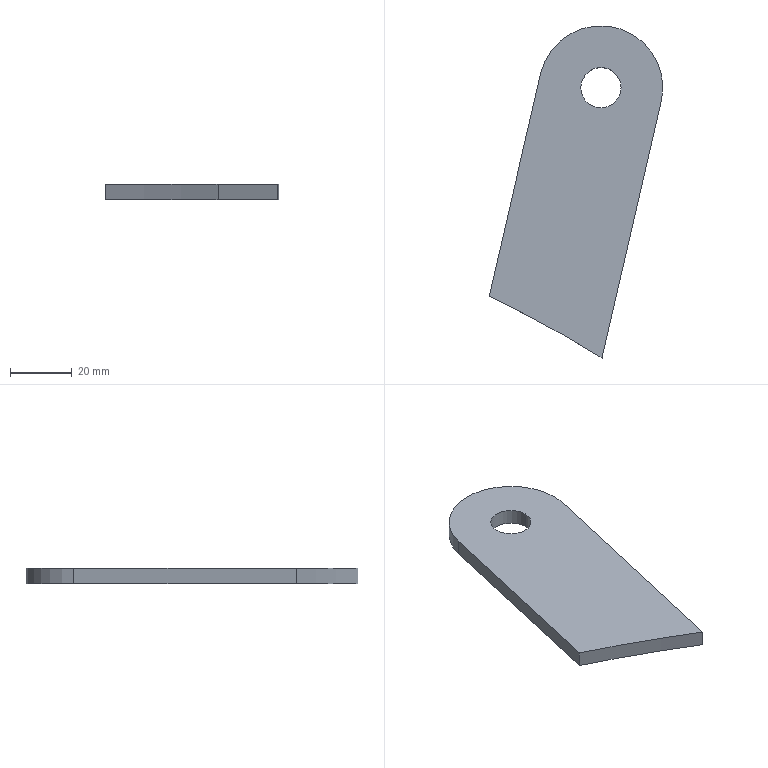Part | SolidWorks | features Extrusion 1 | 1 solid | 8 faces | box 56.087 x 107.32 x 5 mm | volume 18280 mm3 | cylinder 4 | plane 4 | commonest cylinder face diameters 13 x2 40 x1 775 x1
STEP:
#1=CARTESIAN_POINT('',(196.9,416.919,2.5));
#2=VERTEX_POINT('',#1);
#3=CARTESIAN_POINT('',(209.9,416.919,2.5));
#4=VERTEX_POINT('',#3);
#5=CARTESIAN_POINT('',(203.4,416.919,2.5));
#6=DIRECTION('',(0.,0.,1.));
#7=DIRECTION('',(1.,0.,0.));
#8=AXIS2_PLACEMENT_3D('',#5,#6,#7);
#9=CIRCLE('',#8,6.5);
#10=EDGE_CURVE('',#2,#4,#9,.T.);
#11=ORIENTED_EDGE('',*,*,#10,.T.);
#12=CARTESIAN_POINT('',(209.9,416.919,-2.5));
#13=VERTEX_POINT('',#12);
#14=CARTESIAN_POINT('',(209.9,416.919,2.5));
#15=DIRECTION('',(0.,0.,-1.));
#16=VECTOR('',#15,1000.);
#17=LINE('',#14,#16);
#18=EDGE_CURVE('',#4,#13,#17,.T.);
#19=ORIENTED_EDGE('',*,*,#18,.T.);
#20=CARTESIAN_POINT('',(196.9,416.919,-2.5));
#21=VERTEX_POINT('',#20);
#22=CARTESIAN_POINT('',(203.4,416.919,-2.5));
#23=DIRECTION('',(0.,0.,1.));
#24=DIRECTION('',(1.,0.,0.));
#25=AXIS2_PLACEMENT_3D('',#22,#23,#24);
#26=CIRCLE('',#25,6.5);
#27=EDGE_CURVE('',#21,#13,#26,.T.);
#28=ORIENTED_EDGE('',*,*,#27,.F.);
#29=CARTESIAN_POINT('',(196.9,416.919,2.5));
#30=DIRECTION('',(0.,0.,-1.));
#31=VECTOR('',#30,1000.);
#32=LINE('',#29,#31);
#33=EDGE_CURVE('',#2,#21,#32,.T.);
#34=ORIENTED_EDGE('',*,*,#33,.F.);
#35=EDGE_LOOP('',(#11,#19,#28,#34));
#36=FACE_OUTER_BOUND('',#35,.T.);
#37=CARTESIAN_POINT('',(203.4,416.919,2.5));
#38=DIRECTION('',(0.,0.,-1.));
#39=DIRECTION('',(-1.,0.,0.));
#40=AXIS2_PLACEMENT_3D('',#37,#38,#39);
#41=CYLINDRICAL_SURFACE('',#40,6.5);
#42=ADVANCED_FACE('',(#36),#41,.F.);
#43=CARTESIAN_POINT('',(167.313,349.518,2.5));
#44=VERTEX_POINT('',#43);
#45=CARTESIAN_POINT('',(203.767,329.599,2.5));
#46=VERTEX_POINT('',#45);
#47=CARTESIAN_POINT('',(0.,0.,2.5));
#48=DIRECTION('',(0.,0.,-1.));
#49=DIRECTION('',(-1.,0.,0.));
#50=AXIS2_PLACEMENT_3D('',#47,#48,#49);
#51=CIRCLE('',#50,387.5);
#52=EDGE_CURVE('',#44,#46,#51,.T.);
#53=ORIENTED_EDGE('',*,*,#52,.T.);
#54=CARTESIAN_POINT('',(222.887,412.42,2.5));
#55=VERTEX_POINT('',#54);
#56=CARTESIAN_POINT('',(203.767,329.599,2.5));
#57=DIRECTION('',(0.225,0.9744,0.));
#58=VECTOR('',#57,1000.);
#59=LINE('',#56,#58);
#60=EDGE_CURVE('',#46,#55,#59,.T.);
#61=ORIENTED_EDGE('',*,*,#60,.T.);
#62=CARTESIAN_POINT('',(183.913,421.418,2.5));
#63=VERTEX_POINT('',#62);
#64=CARTESIAN_POINT('',(203.4,416.919,2.5));
#65=DIRECTION('',(0.,0.,1.));
#66=DIRECTION('',(-1.,0.,0.));
#67=AXIS2_PLACEMENT_3D('',#64,#65,#66);
#68=CIRCLE('',#67,20.);
#69=EDGE_CURVE('',#55,#63,#68,.T.);
#70=ORIENTED_EDGE('',*,*,#69,.T.);
#71=CARTESIAN_POINT('',(167.313,349.518,2.5));
#72=DIRECTION('',(-0.225,-0.9744,0.));
#73=VECTOR('',#72,1000.);
#74=LINE('',#71,#73);
#75=EDGE_CURVE('',#63,#44,#74,.T.);
#76=ORIENTED_EDGE('',*,*,#75,.T.);
#77=EDGE_LOOP('',(#53,#61,#70,#76));
#78=FACE_OUTER_BOUND('',#77,.T.);
#79=ORIENTED_EDGE('',*,*,#10,.F.);
#80=CARTESIAN_POINT('',(203.4,416.919,2.5));
#81=DIRECTION('',(0.,0.,1.));
#82=DIRECTION('',(1.,0.,0.));
#83=AXIS2_PLACEMENT_3D('',#80,#81,#82);
#84=CIRCLE('',#83,6.5);
#85=EDGE_CURVE('',#4,#2,#84,.T.);
#86=ORIENTED_EDGE('',*,*,#85,.F.);
#87=EDGE_LOOP('',(#79,#86));
#88=FACE_BOUND('',#87,.T.);
#89=CARTESIAN_POINT('',(0.,0.,2.5));
#90=DIRECTION('',(0.,0.,-1.));
#91=DIRECTION('',(-1.,0.,0.));
#92=AXIS2_PLACEMENT_3D('',#89,#90,#91);
#93=PLANE('',#92);
#94=ADVANCED_FACE('',(#78,#88),#93,.F.);
#95=CARTESIAN_POINT('',(167.313,349.518,-2.5));
#96=VERTEX_POINT('',#95);
#97=CARTESIAN_POINT('',(203.767,329.599,-2.5));
#98=VERTEX_POINT('',#97);
#99=CARTESIAN_POINT('',(0.,0.,-2.5));
#100=DIRECTION('',(0.,0.,-1.));
#101=DIRECTION('',(-1.,0.,0.));
#102=AXIS2_PLACEMENT_3D('',#99,#100,#101);
#103=CIRCLE('',#102,387.5);
#104=EDGE_CURVE('',#96,#98,#103,.T.);
#105=ORIENTED_EDGE('',*,*,#104,.F.);
#106=CARTESIAN_POINT('',(183.913,421.418,-2.5));
#107=VERTEX_POINT('',#106);
#108=CARTESIAN_POINT('',(167.313,349.518,-2.5));
#109=DIRECTION('',(-0.225,-0.9744,0.));
#110=VECTOR('',#109,1000.);
#111=LINE('',#108,#110);
#112=EDGE_CURVE('',#107,#96,#111,.T.);
#113=ORIENTED_EDGE('',*,*,#112,.F.);
#114=CARTESIAN_POINT('',(222.887,412.42,-2.5));
#115=VERTEX_POINT('',#114);
#116=CARTESIAN_POINT('',(203.4,416.919,-2.5));
#117=DIRECTION('',(0.,0.,1.));
#118=DIRECTION('',(-1.,0.,0.));
#119=AXIS2_PLACEMENT_3D('',#116,#117,#118);
#120=CIRCLE('',#119,20.);
#121=EDGE_CURVE('',#115,#107,#120,.T.);
#122=ORIENTED_EDGE('',*,*,#121,.F.);
#123=CARTESIAN_POINT('',(203.767,329.599,-2.5));
#124=DIRECTION('',(0.225,0.9744,0.));
#125=VECTOR('',#124,1000.);
#126=LINE('',#123,#125);
#127=EDGE_CURVE('',#98,#115,#126,.T.);
#128=ORIENTED_EDGE('',*,*,#127,.F.);
#129=EDGE_LOOP('',(#105,#113,#122,#128));
#130=FACE_OUTER_BOUND('',#129,.T.);
#131=ORIENTED_EDGE('',*,*,#27,.T.);
#132=CARTESIAN_POINT('',(203.4,416.919,-2.5));
#133=DIRECTION('',(0.,0.,1.));
#134=DIRECTION('',(1.,0.,0.));
#135=AXIS2_PLACEMENT_3D('',#132,#133,#134);
#136=CIRCLE('',#135,6.5);
#137=EDGE_CURVE('',#13,#21,#136,.T.);
#138=ORIENTED_EDGE('',*,*,#137,.T.);
#139=EDGE_LOOP('',(#131,#138));
#140=FACE_BOUND('',#139,.T.);
#141=CARTESIAN_POINT('',(0.,0.,-2.5));
#142=DIRECTION('',(0.,0.,-1.));
#143=DIRECTION('',(-1.,0.,0.));
#144=AXIS2_PLACEMENT_3D('',#141,#142,#143);
#145=PLANE('',#144);
#146=ADVANCED_FACE('',(#130,#140),#145,.T.);
#147=ORIENTED_EDGE('',*,*,#104,.T.);
#148=CARTESIAN_POINT('',(203.767,329.599,2.5));
#149=DIRECTION('',(0.,0.,-1.));
#150=VECTOR('',#149,1000.);
#151=LINE('',#148,#150);
#152=EDGE_CURVE('',#46,#98,#151,.T.);
#153=ORIENTED_EDGE('',*,*,#152,.F.);
#154=ORIENTED_EDGE('',*,*,#52,.F.);
#155=CARTESIAN_POINT('',(167.313,349.518,2.5));
#156=DIRECTION('',(0.,0.,-1.));
#157=VECTOR('',#156,1000.);
#158=LINE('',#155,#157);
#159=EDGE_CURVE('',#44,#96,#158,.T.);
#160=ORIENTED_EDGE('',*,*,#159,.T.);
#161=EDGE_LOOP('',(#147,#153,#154,#160));
#162=FACE_OUTER_BOUND('',#161,.T.);
#163=CARTESIAN_POINT('',(0.,0.,2.5));
#164=DIRECTION('',(0.,0.,-1.));
#165=DIRECTION('',(-1.,0.,0.));
#166=AXIS2_PLACEMENT_3D('',#163,#164,#165);
#167=CYLINDRICAL_SURFACE('',#166,387.5);
#168=ADVANCED_FACE('',(#162),#167,.F.);
#169=ORIENTED_EDGE('',*,*,#127,.T.);
#170=CARTESIAN_POINT('',(222.887,412.42,2.5));
#171=DIRECTION('',(0.,0.,-1.));
#172=VECTOR('',#171,1000.);
#173=LINE('',#170,#172);
#174=EDGE_CURVE('',#55,#115,#173,.T.);
#175=ORIENTED_EDGE('',*,*,#174,.F.);
#176=ORIENTED_EDGE('',*,*,#60,.F.);
#177=ORIENTED_EDGE('',*,*,#152,.T.);
#178=EDGE_LOOP('',(#169,#175,#176,#177));
#179=FACE_OUTER_BOUND('',#178,.T.);
#180=CARTESIAN_POINT('',(203.767,329.599,2.5));
#181=DIRECTION('',(-0.9744,0.225,0.));
#182=DIRECTION('',(-0.225,-0.9744,0.));
#183=AXIS2_PLACEMENT_3D('',#180,#181,#182);
#184=PLANE('',#183);
#185=ADVANCED_FACE('',(#179),#184,.F.);
#186=ORIENTED_EDGE('',*,*,#121,.T.);
#187=CARTESIAN_POINT('',(183.913,421.418,2.5));
#188=DIRECTION('',(0.,0.,-1.));
#189=VECTOR('',#188,1000.);
#190=LINE('',#187,#189);
#191=EDGE_CURVE('',#63,#107,#190,.T.);
#192=ORIENTED_EDGE('',*,*,#191,.F.);
#193=ORIENTED_EDGE('',*,*,#69,.F.);
#194=ORIENTED_EDGE('',*,*,#174,.T.);
#195=EDGE_LOOP('',(#186,#192,#193,#194));
#196=FACE_OUTER_BOUND('',#195,.T.);
#197=CARTESIAN_POINT('',(203.4,416.919,2.5));
#198=DIRECTION('',(0.,0.,-1.));
#199=DIRECTION('',(-1.,0.,0.));
#200=AXIS2_PLACEMENT_3D('',#197,#198,#199);
#201=CYLINDRICAL_SURFACE('',#200,20.);
#202=ADVANCED_FACE('',(#196),#201,.T.);
#203=ORIENTED_EDGE('',*,*,#112,.T.);
#204=ORIENTED_EDGE('',*,*,#159,.F.);
#205=ORIENTED_EDGE('',*,*,#75,.F.);
#206=ORIENTED_EDGE('',*,*,#191,.T.);
#207=EDGE_LOOP('',(#203,#204,#205,#206));
#208=FACE_OUTER_BOUND('',#207,.T.);
#209=CARTESIAN_POINT('',(167.313,349.518,2.5));
#210=DIRECTION('',(0.9744,-0.225,0.));
#211=DIRECTION('',(0.225,0.9744,0.));
#212=AXIS2_PLACEMENT_3D('',#209,#210,#211);
#213=PLANE('',#212);
#214=ADVANCED_FACE('',(#208),#213,.F.);
#215=ORIENTED_EDGE('',*,*,#18,.F.);
#216=ORIENTED_EDGE('',*,*,#85,.T.);
#217=ORIENTED_EDGE('',*,*,#33,.T.);
#218=ORIENTED_EDGE('',*,*,#137,.F.);
#219=EDGE_LOOP('',(#215,#216,#217,#218));
#220=FACE_OUTER_BOUND('',#219,.T.);
#221=CARTESIAN_POINT('',(203.4,416.919,2.5));
#222=DIRECTION('',(0.,0.,-1.));
#223=DIRECTION('',(-1.,0.,0.));
#224=AXIS2_PLACEMENT_3D('',#221,#222,#223);
#225=CYLINDRICAL_SURFACE('',#224,6.5);
#226=ADVANCED_FACE('',(#220),#225,.F.);
#227=CLOSED_SHELL('',(#42,#94,#146,#168,#185,#202,#214,#226));
#228=MANIFOLD_SOLID_BREP('',#227);
#229=CARTESIAN_POINT('',(0.,0.,0.));
#230=DIRECTION('',(0.,0.,1.));
#231=DIRECTION('',(1.,0.,0.));
#232=AXIS2_PLACEMENT_3D('',#229,#230,#231);
#233=(LENGTH_UNIT()NAMED_UNIT(*)SI_UNIT(.MILLI.,.METRE.));
#234=UNCERTAINTY_MEASURE_WITH_UNIT(LENGTH_MEASURE(0.00001),#233,'','');
#235=(NAMED_UNIT(*)PLANE_ANGLE_UNIT()SI_UNIT($,.RADIAN.));
#236=(NAMED_UNIT(*)SI_UNIT($,.STERADIAN.)SOLID_ANGLE_UNIT());
#237=(GEOMETRIC_REPRESENTATION_CONTEXT(3)GLOBAL_UNCERTAINTY_ASSIGNED_CONTEXT((#234))GLOBAL_UNIT_ASSIGNED_CONTEXT((#233,#235,#236))REPRESENTATION_CONTEXT('',''));
#238=ADVANCED_BREP_SHAPE_REPRESENTATION('',(#228,#232),#237);